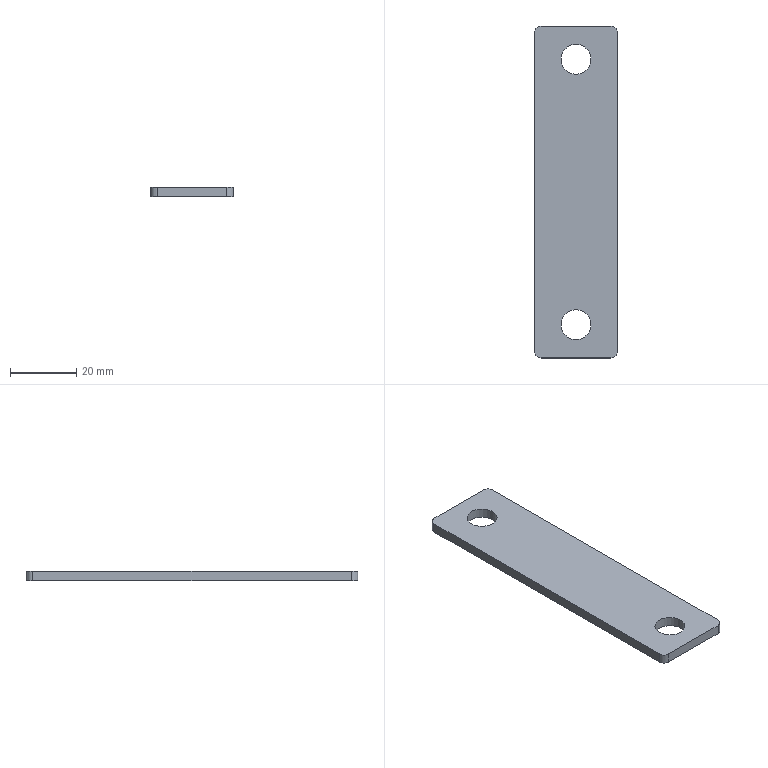Part | STEP file | 7471302 | 1 solid | 12 faces | box 25 x 100 x 3 mm | volume 7108 mm3 | cylinder 6 | plane 6 | commonest cylinder face diameters 4 x4 9 x2
STEP:
#1=CARTESIAN_POINT('',(0.,0.,0.));
#2=DIRECTION('',(0.,0.,1.));
#3=DIRECTION('',(1.,0.,0.));
#4=AXIS2_PLACEMENT_3D('',#1,#2,#3);
#5=CARTESIAN_POINT('',(15.714,-68.195,0.));
#6=VERTEX_POINT('',#5);
#7=CARTESIAN_POINT('',(17.714,-66.195,0.));
#8=VERTEX_POINT('',#7);
#9=CARTESIAN_POINT('',(15.714,-66.195,0.));
#10=DIRECTION('',(0.,0.,1.));
#11=DIRECTION('',(1.,0.,0.));
#12=AXIS2_PLACEMENT_3D('',#9,#10,#11);
#13=CIRCLE('',#12,2.);
#14=CARTESIAN_POINT('',(15.714,-66.195,3.));
#15=DIRECTION('',(0.,0.,-1.));
#16=DIRECTION('',(-1.,0.,0.));
#17=AXIS2_PLACEMENT_3D('',#14,#15,#16);
#18=CYLINDRICAL_SURFACE('',#17,2.);
#19=CARTESIAN_POINT('',(9.425,3.));
#20=DIRECTION('',(-1.,0.));
#21=VECTOR('',#20,1.);
#22=LINE('',#19,#21);
#23=(GEOMETRIC_REPRESENTATION_CONTEXT(2)PARAMETRIC_REPRESENTATION_CONTEXT()REPRESENTATION_CONTEXT('',''));
#24=DEFINITIONAL_REPRESENTATION('',(#22),#23);
#25=PCURVE('',#18,#24);
#26=CARTESIAN_POINT('',(15.714,-66.195,0.));
#27=DIRECTION('',(0.,0.,1.));
#28=DIRECTION('',(1.,0.,0.));
#29=AXIS2_PLACEMENT_3D('',#26,#27,#28);
#30=PLANE('',#29);
#31=CARTESIAN_POINT('',(0.,0.));
#32=DIRECTION('',(1.,0.));
#33=AXIS2_PLACEMENT_2D('',#31,#32);
#34=CIRCLE('',#33,2.);
#35=(GEOMETRIC_REPRESENTATION_CONTEXT(2)PARAMETRIC_REPRESENTATION_CONTEXT()REPRESENTATION_CONTEXT('',''));
#36=DEFINITIONAL_REPRESENTATION('',(#34),#35);
#37=PCURVE('',#30,#36);
#38=SURFACE_CURVE('',#13,(#25,#37),.PCURVE_S1.);
#39=EDGE_CURVE('',#6,#8,#38,.T.);
#40=ORIENTED_EDGE('',*,*,#39,.T.);
#41=CARTESIAN_POINT('',(17.714,-66.195,3.));
#42=VERTEX_POINT('',#41);
#43=CARTESIAN_POINT('',(17.714,-66.195,3.));
#44=DIRECTION('',(0.,0.,-1.));
#45=VECTOR('',#44,1.);
#46=LINE('',#43,#45);
#47=CARTESIAN_POINT('',(3.142,0.));
#48=DIRECTION('',(0.,1.));
#49=VECTOR('',#48,1.);
#50=LINE('',#47,#49);
#51=(GEOMETRIC_REPRESENTATION_CONTEXT(2)PARAMETRIC_REPRESENTATION_CONTEXT()REPRESENTATION_CONTEXT('',''));
#52=DEFINITIONAL_REPRESENTATION('',(#50),#51);
#53=PCURVE('',#18,#52);
#54=CARTESIAN_POINT('',(17.714,29.805,3.));
#55=DIRECTION('',(-1.,0.,0.));
#56=DIRECTION('',(0.,-1.,0.));
#57=AXIS2_PLACEMENT_3D('',#54,#55,#56);
#58=PLANE('',#57);
#59=CARTESIAN_POINT('',(96.,0.));
#60=DIRECTION('',(0.,-1.));
#61=VECTOR('',#60,1.);
#62=LINE('',#59,#61);
#63=(GEOMETRIC_REPRESENTATION_CONTEXT(2)PARAMETRIC_REPRESENTATION_CONTEXT()REPRESENTATION_CONTEXT('',''));
#64=DEFINITIONAL_REPRESENTATION('',(#62),#63);
#65=PCURVE('',#58,#64);
#66=SURFACE_CURVE('',#46,(#53,#65),.PCURVE_S1.);
#67=EDGE_CURVE('',#42,#8,#66,.T.);
#68=ORIENTED_EDGE('',*,*,#67,.F.);
#69=CARTESIAN_POINT('',(15.714,-68.195,3.));
#70=VERTEX_POINT('',#69);
#71=CARTESIAN_POINT('',(15.714,-66.195,3.));
#72=DIRECTION('',(0.,0.,1.));
#73=DIRECTION('',(1.,0.,0.));
#74=AXIS2_PLACEMENT_3D('',#71,#72,#73);
#75=CIRCLE('',#74,2.);
#76=CARTESIAN_POINT('',(9.425,0.));
#77=DIRECTION('',(-1.,0.));
#78=VECTOR('',#77,1.);
#79=LINE('',#76,#78);
#80=(GEOMETRIC_REPRESENTATION_CONTEXT(2)PARAMETRIC_REPRESENTATION_CONTEXT()REPRESENTATION_CONTEXT('',''));
#81=DEFINITIONAL_REPRESENTATION('',(#79),#80);
#82=PCURVE('',#18,#81);
#83=CARTESIAN_POINT('',(15.714,-66.195,3.));
#84=DIRECTION('',(0.,0.,1.));
#85=DIRECTION('',(1.,0.,0.));
#86=AXIS2_PLACEMENT_3D('',#83,#84,#85);
#87=PLANE('',#86);
#88=CARTESIAN_POINT('',(0.,0.));
#89=DIRECTION('',(1.,0.));
#90=AXIS2_PLACEMENT_2D('',#88,#89);
#91=CIRCLE('',#90,2.);
#92=(GEOMETRIC_REPRESENTATION_CONTEXT(2)PARAMETRIC_REPRESENTATION_CONTEXT()REPRESENTATION_CONTEXT('',''));
#93=DEFINITIONAL_REPRESENTATION('',(#91),#92);
#94=PCURVE('',#87,#93);
#95=SURFACE_CURVE('',#75,(#82,#94),.PCURVE_S1.);
#96=EDGE_CURVE('',#70,#42,#95,.T.);
#97=ORIENTED_EDGE('',*,*,#96,.F.);
#98=CARTESIAN_POINT('',(15.714,-68.195,3.));
#99=DIRECTION('',(0.,0.,-1.));
#100=VECTOR('',#99,1.);
#101=LINE('',#98,#100);
#102=CARTESIAN_POINT('',(4.712,0.));
#103=DIRECTION('',(0.,1.));
#104=VECTOR('',#103,1.);
#105=LINE('',#102,#104);
#106=(GEOMETRIC_REPRESENTATION_CONTEXT(2)PARAMETRIC_REPRESENTATION_CONTEXT()REPRESENTATION_CONTEXT('',''));
#107=DEFINITIONAL_REPRESENTATION('',(#105),#106);
#108=PCURVE('',#18,#107);
#109=CARTESIAN_POINT('',(-5.286,-68.195,3.));
#110=DIRECTION('',(0.,1.,0.));
#111=DIRECTION('',(0.,0.,1.));
#112=AXIS2_PLACEMENT_3D('',#109,#110,#111);
#113=PLANE('',#112);
#114=CARTESIAN_POINT('',(0.,21.));
#115=DIRECTION('',(-1.,0.));
#116=VECTOR('',#115,1.);
#117=LINE('',#114,#116);
#118=(GEOMETRIC_REPRESENTATION_CONTEXT(2)PARAMETRIC_REPRESENTATION_CONTEXT()REPRESENTATION_CONTEXT('',''));
#119=DEFINITIONAL_REPRESENTATION('',(#117),#118);
#120=PCURVE('',#113,#119);
#121=SURFACE_CURVE('',#101,(#108,#120),.PCURVE_S1.);
#122=EDGE_CURVE('',#70,#6,#121,.T.);
#123=ORIENTED_EDGE('',*,*,#122,.T.);
#124=EDGE_LOOP('',(#40,#68,#97,#123));
#125=FACE_BOUND('',#124,.T.);
#126=ADVANCED_FACE('',(#125),#18,.T.);
#127=CARTESIAN_POINT('',(17.714,29.805,0.));
#128=VERTEX_POINT('',#127);
#129=CARTESIAN_POINT('',(17.714,29.805,0.));
#130=DIRECTION('',(0.,1.,0.));
#131=VECTOR('',#130,1.);
#132=LINE('',#129,#131);
#133=CARTESIAN_POINT('',(0.,-3.));
#134=DIRECTION('',(-1.,0.));
#135=VECTOR('',#134,1.);
#136=LINE('',#133,#135);
#137=(GEOMETRIC_REPRESENTATION_CONTEXT(2)PARAMETRIC_REPRESENTATION_CONTEXT()REPRESENTATION_CONTEXT('',''));
#138=DEFINITIONAL_REPRESENTATION('',(#136),#137);
#139=PCURVE('',#58,#138);
#140=CARTESIAN_POINT('',(2.,96.));
#141=DIRECTION('',(0.,1.));
#142=VECTOR('',#141,1.);
#143=LINE('',#140,#142);
#144=(GEOMETRIC_REPRESENTATION_CONTEXT(2)PARAMETRIC_REPRESENTATION_CONTEXT()REPRESENTATION_CONTEXT('',''));
#145=DEFINITIONAL_REPRESENTATION('',(#143),#144);
#146=PCURVE('',#30,#145);
#147=SURFACE_CURVE('',#132,(#139,#146),.PCURVE_S1.);
#148=EDGE_CURVE('',#8,#128,#147,.T.);
#149=ORIENTED_EDGE('',*,*,#148,.T.);
#150=CARTESIAN_POINT('',(17.714,29.805,3.));
#151=VERTEX_POINT('',#150);
#152=CARTESIAN_POINT('',(17.714,29.805,3.));
#153=DIRECTION('',(0.,0.,-1.));
#154=VECTOR('',#153,1.);
#155=LINE('',#152,#154);
#156=CARTESIAN_POINT('',(0.,0.));
#157=DIRECTION('',(0.,-1.));
#158=VECTOR('',#157,1.);
#159=LINE('',#156,#158);
#160=(GEOMETRIC_REPRESENTATION_CONTEXT(2)PARAMETRIC_REPRESENTATION_CONTEXT()REPRESENTATION_CONTEXT('',''));
#161=DEFINITIONAL_REPRESENTATION('',(#159),#160);
#162=PCURVE('',#58,#161);
#163=CARTESIAN_POINT('',(15.714,29.805,3.));
#164=DIRECTION('',(0.,0.,-1.));
#165=DIRECTION('',(-1.,0.,0.));
#166=AXIS2_PLACEMENT_3D('',#163,#164,#165);
#167=CYLINDRICAL_SURFACE('',#166,2.);
#168=CARTESIAN_POINT('',(3.142,0.));
#169=DIRECTION('',(0.,1.));
#170=VECTOR('',#169,1.);
#171=LINE('',#168,#170);
#172=(GEOMETRIC_REPRESENTATION_CONTEXT(2)PARAMETRIC_REPRESENTATION_CONTEXT()REPRESENTATION_CONTEXT('',''));
#173=DEFINITIONAL_REPRESENTATION('',(#171),#172);
#174=PCURVE('',#167,#173);
#175=SURFACE_CURVE('',#155,(#162,#174),.PCURVE_S1.);
#176=EDGE_CURVE('',#151,#128,#175,.T.);
#177=ORIENTED_EDGE('',*,*,#176,.F.);
#178=CARTESIAN_POINT('',(17.714,29.805,3.));
#179=DIRECTION('',(0.,1.,0.));
#180=VECTOR('',#179,1.);
#181=LINE('',#178,#180);
#182=CARTESIAN_POINT('',(0.,0.));
#183=DIRECTION('',(-1.,0.));
#184=VECTOR('',#183,1.);
#185=LINE('',#182,#184);
#186=(GEOMETRIC_REPRESENTATION_CONTEXT(2)PARAMETRIC_REPRESENTATION_CONTEXT()REPRESENTATION_CONTEXT('',''));
#187=DEFINITIONAL_REPRESENTATION('',(#185),#186);
#188=PCURVE('',#58,#187);
#189=CARTESIAN_POINT('',(2.,96.));
#190=DIRECTION('',(0.,1.));
#191=VECTOR('',#190,1.);
#192=LINE('',#189,#191);
#193=(GEOMETRIC_REPRESENTATION_CONTEXT(2)PARAMETRIC_REPRESENTATION_CONTEXT()REPRESENTATION_CONTEXT('',''));
#194=DEFINITIONAL_REPRESENTATION('',(#192),#193);
#195=PCURVE('',#87,#194);
#196=SURFACE_CURVE('',#181,(#188,#195),.PCURVE_S1.);
#197=EDGE_CURVE('',#42,#151,#196,.T.);
#198=ORIENTED_EDGE('',*,*,#197,.F.);
#199=ORIENTED_EDGE('',*,*,#67,.T.);
#200=EDGE_LOOP('',(#149,#177,#198,#199));
#201=FACE_BOUND('',#200,.T.);
#202=ADVANCED_FACE('',(#201),#58,.F.);
#203=CARTESIAN_POINT('',(15.714,31.805,0.));
#204=VERTEX_POINT('',#203);
#205=CARTESIAN_POINT('',(15.714,29.805,0.));
#206=DIRECTION('',(0.,0.,1.));
#207=DIRECTION('',(-1.,0.,0.));
#208=AXIS2_PLACEMENT_3D('',#205,#206,#207);
#209=CIRCLE('',#208,2.);
#210=CARTESIAN_POINT('',(6.283,3.));
#211=DIRECTION('',(-1.,0.));
#212=VECTOR('',#211,1.);
#213=LINE('',#210,#212);
#214=(GEOMETRIC_REPRESENTATION_CONTEXT(2)PARAMETRIC_REPRESENTATION_CONTEXT()REPRESENTATION_CONTEXT('',''));
#215=DEFINITIONAL_REPRESENTATION('',(#213),#214);
#216=PCURVE('',#167,#215);
#217=CARTESIAN_POINT('',(0.,96.));
#218=DIRECTION('',(-1.,0.));
#219=AXIS2_PLACEMENT_2D('',#217,#218);
#220=CIRCLE('',#219,2.);
#221=(GEOMETRIC_REPRESENTATION_CONTEXT(2)PARAMETRIC_REPRESENTATION_CONTEXT()REPRESENTATION_CONTEXT('',''));
#222=DEFINITIONAL_REPRESENTATION('',(#220),#221);
#223=PCURVE('',#30,#222);
#224=SURFACE_CURVE('',#209,(#216,#223),.PCURVE_S1.);
#225=EDGE_CURVE('',#128,#204,#224,.T.);
#226=ORIENTED_EDGE('',*,*,#225,.T.);
#227=CARTESIAN_POINT('',(15.714,31.805,3.));
#228=VERTEX_POINT('',#227);
#229=CARTESIAN_POINT('',(15.714,31.805,3.));
#230=DIRECTION('',(0.,0.,-1.));
#231=VECTOR('',#230,1.);
#232=LINE('',#229,#231);
#233=CARTESIAN_POINT('',(1.571,0.));
#234=DIRECTION('',(0.,1.));
#235=VECTOR('',#234,1.);
#236=LINE('',#233,#235);
#237=(GEOMETRIC_REPRESENTATION_CONTEXT(2)PARAMETRIC_REPRESENTATION_CONTEXT()REPRESENTATION_CONTEXT('',''));
#238=DEFINITIONAL_REPRESENTATION('',(#236),#237);
#239=PCURVE('',#167,#238);
#240=CARTESIAN_POINT('',(-5.286,31.805,3.));
#241=DIRECTION('',(0.,-1.,0.));
#242=DIRECTION('',(0.,0.,-1.));
#243=AXIS2_PLACEMENT_3D('',#240,#241,#242);
#244=PLANE('',#243);
#245=CARTESIAN_POINT('',(0.,21.));
#246=DIRECTION('',(1.,0.));
#247=VECTOR('',#246,1.);
#248=LINE('',#245,#247);
#249=(GEOMETRIC_REPRESENTATION_CONTEXT(2)PARAMETRIC_REPRESENTATION_CONTEXT()REPRESENTATION_CONTEXT('',''));
#250=DEFINITIONAL_REPRESENTATION('',(#248),#249);
#251=PCURVE('',#244,#250);
#252=SURFACE_CURVE('',#232,(#239,#251),.PCURVE_S1.);
#253=EDGE_CURVE('',#228,#204,#252,.T.);
#254=ORIENTED_EDGE('',*,*,#253,.F.);
#255=CARTESIAN_POINT('',(15.714,29.805,3.));
#256=DIRECTION('',(0.,0.,1.));
#257=DIRECTION('',(-1.,0.,0.));
#258=AXIS2_PLACEMENT_3D('',#255,#256,#257);
#259=CIRCLE('',#258,2.);
#260=CARTESIAN_POINT('',(6.283,0.));
#261=DIRECTION('',(-1.,0.));
#262=VECTOR('',#261,1.);
#263=LINE('',#260,#262);
#264=(GEOMETRIC_REPRESENTATION_CONTEXT(2)PARAMETRIC_REPRESENTATION_CONTEXT()REPRESENTATION_CONTEXT('',''));
#265=DEFINITIONAL_REPRESENTATION('',(#263),#264);
#266=PCURVE('',#167,#265);
#267=CARTESIAN_POINT('',(0.,96.));
#268=DIRECTION('',(-1.,0.));
#269=AXIS2_PLACEMENT_2D('',#267,#268);
#270=CIRCLE('',#269,2.);
#271=(GEOMETRIC_REPRESENTATION_CONTEXT(2)PARAMETRIC_REPRESENTATION_CONTEXT()REPRESENTATION_CONTEXT('',''));
#272=DEFINITIONAL_REPRESENTATION('',(#270),#271);
#273=PCURVE('',#87,#272);
#274=SURFACE_CURVE('',#259,(#266,#273),.PCURVE_S1.);
#275=EDGE_CURVE('',#151,#228,#274,.T.);
#276=ORIENTED_EDGE('',*,*,#275,.F.);
#277=ORIENTED_EDGE('',*,*,#176,.T.);
#278=EDGE_LOOP('',(#226,#254,#276,#277));
#279=FACE_BOUND('',#278,.T.);
#280=ADVANCED_FACE('',(#279),#167,.T.);
#281=CARTESIAN_POINT('',(-5.286,31.805,0.));
#282=VERTEX_POINT('',#281);
#283=CARTESIAN_POINT('',(-5.286,31.805,0.));
#284=DIRECTION('',(-1.,0.,0.));
#285=VECTOR('',#284,1.);
#286=LINE('',#283,#285);
#287=CARTESIAN_POINT('',(3.,0.));
#288=DIRECTION('',(0.,-1.));
#289=VECTOR('',#288,1.);
#290=LINE('',#287,#289);
#291=(GEOMETRIC_REPRESENTATION_CONTEXT(2)PARAMETRIC_REPRESENTATION_CONTEXT()REPRESENTATION_CONTEXT('',''));
#292=DEFINITIONAL_REPRESENTATION('',(#290),#291);
#293=PCURVE('',#244,#292);
#294=CARTESIAN_POINT('',(-21.,98.));
#295=DIRECTION('',(-1.,0.));
#296=VECTOR('',#295,1.);
#297=LINE('',#294,#296);
#298=(GEOMETRIC_REPRESENTATION_CONTEXT(2)PARAMETRIC_REPRESENTATION_CONTEXT()REPRESENTATION_CONTEXT('',''));
#299=DEFINITIONAL_REPRESENTATION('',(#297),#298);
#300=PCURVE('',#30,#299);
#301=SURFACE_CURVE('',#286,(#293,#300),.PCURVE_S1.);
#302=EDGE_CURVE('',#204,#282,#301,.T.);
#303=ORIENTED_EDGE('',*,*,#302,.T.);
#304=CARTESIAN_POINT('',(-5.286,31.805,3.));
#305=VERTEX_POINT('',#304);
#306=CARTESIAN_POINT('',(-5.286,31.805,3.));
#307=DIRECTION('',(0.,0.,-1.));
#308=VECTOR('',#307,1.);
#309=LINE('',#306,#308);
#310=CARTESIAN_POINT('',(0.,0.));
#311=DIRECTION('',(1.,0.));
#312=VECTOR('',#311,1.);
#313=LINE('',#310,#312);
#314=(GEOMETRIC_REPRESENTATION_CONTEXT(2)PARAMETRIC_REPRESENTATION_CONTEXT()REPRESENTATION_CONTEXT('',''));
#315=DEFINITIONAL_REPRESENTATION('',(#313),#314);
#316=PCURVE('',#244,#315);
#317=CARTESIAN_POINT('',(-5.286,29.805,3.));
#318=DIRECTION('',(0.,0.,-1.));
#319=DIRECTION('',(-1.,0.,0.));
#320=AXIS2_PLACEMENT_3D('',#317,#318,#319);
#321=CYLINDRICAL_SURFACE('',#320,2.);
#322=CARTESIAN_POINT('',(1.571,0.));
#323=DIRECTION('',(0.,1.));
#324=VECTOR('',#323,1.);
#325=LINE('',#322,#324);
#326=(GEOMETRIC_REPRESENTATION_CONTEXT(2)PARAMETRIC_REPRESENTATION_CONTEXT()REPRESENTATION_CONTEXT('',''));
#327=DEFINITIONAL_REPRESENTATION('',(#325),#326);
#328=PCURVE('',#321,#327);
#329=SURFACE_CURVE('',#309,(#316,#328),.PCURVE_S1.);
#330=EDGE_CURVE('',#305,#282,#329,.T.);
#331=ORIENTED_EDGE('',*,*,#330,.F.);
#332=CARTESIAN_POINT('',(-5.286,31.805,3.));
#333=DIRECTION('',(-1.,0.,0.));
#334=VECTOR('',#333,1.);
#335=LINE('',#332,#334);
#336=CARTESIAN_POINT('',(0.,0.));
#337=DIRECTION('',(0.,-1.));
#338=VECTOR('',#337,1.);
#339=LINE('',#336,#338);
#340=(GEOMETRIC_REPRESENTATION_CONTEXT(2)PARAMETRIC_REPRESENTATION_CONTEXT()REPRESENTATION_CONTEXT('',''));
#341=DEFINITIONAL_REPRESENTATION('',(#339),#340);
#342=PCURVE('',#244,#341);
#343=CARTESIAN_POINT('',(-21.,98.));
#344=DIRECTION('',(-1.,0.));
#345=VECTOR('',#344,1.);
#346=LINE('',#343,#345);
#347=(GEOMETRIC_REPRESENTATION_CONTEXT(2)PARAMETRIC_REPRESENTATION_CONTEXT()REPRESENTATION_CONTEXT('',''));
#348=DEFINITIONAL_REPRESENTATION('',(#346),#347);
#349=PCURVE('',#87,#348);
#350=SURFACE_CURVE('',#335,(#342,#349),.PCURVE_S1.);
#351=EDGE_CURVE('',#228,#305,#350,.T.);
#352=ORIENTED_EDGE('',*,*,#351,.F.);
#353=ORIENTED_EDGE('',*,*,#253,.T.);
#354=EDGE_LOOP('',(#303,#331,#352,#353));
#355=FACE_BOUND('',#354,.T.);
#356=ADVANCED_FACE('',(#355),#244,.F.);
#357=CARTESIAN_POINT('',(-7.286,29.805,0.));
#358=VERTEX_POINT('',#357);
#359=CARTESIAN_POINT('',(-5.286,29.805,0.));
#360=DIRECTION('',(0.,0.,1.));
#361=DIRECTION('',(1.,0.,0.));
#362=AXIS2_PLACEMENT_3D('',#359,#360,#361);
#363=CIRCLE('',#362,2.);
#364=CARTESIAN_POINT('',(3.142,3.));
#365=DIRECTION('',(-1.,0.));
#366=VECTOR('',#365,1.);
#367=LINE('',#364,#366);
#368=(GEOMETRIC_REPRESENTATION_CONTEXT(2)PARAMETRIC_REPRESENTATION_CONTEXT()REPRESENTATION_CONTEXT('',''));
#369=DEFINITIONAL_REPRESENTATION('',(#367),#368);
#370=PCURVE('',#321,#369);
#371=CARTESIAN_POINT('',(-21.,96.));
#372=DIRECTION('',(1.,0.));
#373=AXIS2_PLACEMENT_2D('',#371,#372);
#374=CIRCLE('',#373,2.);
#375=(GEOMETRIC_REPRESENTATION_CONTEXT(2)PARAMETRIC_REPRESENTATION_CONTEXT()REPRESENTATION_CONTEXT('',''));
#376=DEFINITIONAL_REPRESENTATION('',(#374),#375);
#377=PCURVE('',#30,#376);
#378=SURFACE_CURVE('',#363,(#370,#377),.PCURVE_S1.);
#379=EDGE_CURVE('',#282,#358,#378,.T.);
#380=ORIENTED_EDGE('',*,*,#379,.T.);
#381=CARTESIAN_POINT('',(-7.286,29.805,3.));
#382=VERTEX_POINT('',#381);
#383=CARTESIAN_POINT('',(-7.286,29.805,3.));
#384=DIRECTION('',(0.,0.,-1.));
#385=VECTOR('',#384,1.);
#386=LINE('',#383,#385);
#387=CARTESIAN_POINT('',(0.,0.));
#388=DIRECTION('',(0.,1.));
#389=VECTOR('',#388,1.);
#390=LINE('',#387,#389);
#391=(GEOMETRIC_REPRESENTATION_CONTEXT(2)PARAMETRIC_REPRESENTATION_CONTEXT()REPRESENTATION_CONTEXT('',''));
#392=DEFINITIONAL_REPRESENTATION('',(#390),#391);
#393=PCURVE('',#321,#392);
#394=CARTESIAN_POINT('',(-7.286,29.805,3.));
#395=DIRECTION('',(1.,0.,0.));
#396=DIRECTION('',(0.,1.,0.));
#397=AXIS2_PLACEMENT_3D('',#394,#395,#396);
#398=PLANE('',#397);
#399=CARTESIAN_POINT('',(0.,0.));
#400=DIRECTION('',(0.,-1.));
#401=VECTOR('',#400,1.);
#402=LINE('',#399,#401);
#403=(GEOMETRIC_REPRESENTATION_CONTEXT(2)PARAMETRIC_REPRESENTATION_CONTEXT()REPRESENTATION_CONTEXT('',''));
#404=DEFINITIONAL_REPRESENTATION('',(#402),#403);
#405=PCURVE('',#398,#404);
#406=SURFACE_CURVE('',#386,(#393,#405),.PCURVE_S1.);
#407=EDGE_CURVE('',#382,#358,#406,.T.);
#408=ORIENTED_EDGE('',*,*,#407,.F.);
#409=CARTESIAN_POINT('',(-5.286,29.805,3.));
#410=DIRECTION('',(0.,0.,1.));
#411=DIRECTION('',(1.,0.,0.));
#412=AXIS2_PLACEMENT_3D('',#409,#410,#411);
#413=CIRCLE('',#412,2.);
#414=CARTESIAN_POINT('',(3.142,0.));
#415=DIRECTION('',(-1.,0.));
#416=VECTOR('',#415,1.);
#417=LINE('',#414,#416);
#418=(GEOMETRIC_REPRESENTATION_CONTEXT(2)PARAMETRIC_REPRESENTATION_CONTEXT()REPRESENTATION_CONTEXT('',''));
#419=DEFINITIONAL_REPRESENTATION('',(#417),#418);
#420=PCURVE('',#321,#419);
#421=CARTESIAN_POINT('',(-21.,96.));
#422=DIRECTION('',(1.,0.));
#423=AXIS2_PLACEMENT_2D('',#421,#422);
#424=CIRCLE('',#423,2.);
#425=(GEOMETRIC_REPRESENTATION_CONTEXT(2)PARAMETRIC_REPRESENTATION_CONTEXT()REPRESENTATION_CONTEXT('',''));
#426=DEFINITIONAL_REPRESENTATION('',(#424),#425);
#427=PCURVE('',#87,#426);
#428=SURFACE_CURVE('',#413,(#420,#427),.PCURVE_S1.);
#429=EDGE_CURVE('',#305,#382,#428,.T.);
#430=ORIENTED_EDGE('',*,*,#429,.F.);
#431=ORIENTED_EDGE('',*,*,#330,.T.);
#432=EDGE_LOOP('',(#380,#408,#430,#431));
#433=FACE_BOUND('',#432,.T.);
#434=ADVANCED_FACE('',(#433),#321,.T.);
#435=CARTESIAN_POINT('',(-7.286,-66.195,0.));
#436=VERTEX_POINT('',#435);
#437=CARTESIAN_POINT('',(-7.286,29.805,0.));
#438=DIRECTION('',(0.,-1.,0.));
#439=VECTOR('',#438,1.);
#440=LINE('',#437,#439);
#441=CARTESIAN_POINT('',(0.,-3.));
#442=DIRECTION('',(-1.,0.));
#443=VECTOR('',#442,1.);
#444=LINE('',#441,#443);
#445=(GEOMETRIC_REPRESENTATION_CONTEXT(2)PARAMETRIC_REPRESENTATION_CONTEXT()REPRESENTATION_CONTEXT('',''));
#446=DEFINITIONAL_REPRESENTATION('',(#444),#445);
#447=PCURVE('',#398,#446);
#448=CARTESIAN_POINT('',(-23.,96.));
#449=DIRECTION('',(0.,-1.));
#450=VECTOR('',#449,1.);
#451=LINE('',#448,#450);
#452=(GEOMETRIC_REPRESENTATION_CONTEXT(2)PARAMETRIC_REPRESENTATION_CONTEXT()REPRESENTATION_CONTEXT('',''));
#453=DEFINITIONAL_REPRESENTATION('',(#451),#452);
#454=PCURVE('',#30,#453);
#455=SURFACE_CURVE('',#440,(#447,#454),.PCURVE_S1.);
#456=EDGE_CURVE('',#358,#436,#455,.T.);
#457=ORIENTED_EDGE('',*,*,#456,.T.);
#458=CARTESIAN_POINT('',(-7.286,-66.195,3.));
#459=VERTEX_POINT('',#458);
#460=CARTESIAN_POINT('',(-7.286,-66.195,3.));
#461=DIRECTION('',(0.,0.,-1.));
#462=VECTOR('',#461,1.);
#463=LINE('',#460,#462);
#464=CARTESIAN_POINT('',(-96.,0.));
#465=DIRECTION('',(0.,-1.));
#466=VECTOR('',#465,1.);
#467=LINE('',#464,#466);
#468=(GEOMETRIC_REPRESENTATION_CONTEXT(2)PARAMETRIC_REPRESENTATION_CONTEXT()REPRESENTATION_CONTEXT('',''));
#469=DEFINITIONAL_REPRESENTATION('',(#467),#468);
#470=PCURVE('',#398,#469);
#471=CARTESIAN_POINT('',(-5.286,-66.195,3.));
#472=DIRECTION('',(0.,0.,-1.));
#473=DIRECTION('',(-1.,0.,0.));
#474=AXIS2_PLACEMENT_3D('',#471,#472,#473);
#475=CYLINDRICAL_SURFACE('',#474,2.);
#476=CARTESIAN_POINT('',(6.283,0.));
#477=DIRECTION('',(0.,1.));
#478=VECTOR('',#477,1.);
#479=LINE('',#476,#478);
#480=(GEOMETRIC_REPRESENTATION_CONTEXT(2)PARAMETRIC_REPRESENTATION_CONTEXT()REPRESENTATION_CONTEXT('',''));
#481=DEFINITIONAL_REPRESENTATION('',(#479),#480);
#482=PCURVE('',#475,#481);
#483=SURFACE_CURVE('',#463,(#470,#482),.PCURVE_S1.);
#484=EDGE_CURVE('',#459,#436,#483,.T.);
#485=ORIENTED_EDGE('',*,*,#484,.F.);
#486=CARTESIAN_POINT('',(-7.286,29.805,3.));
#487=DIRECTION('',(0.,-1.,0.));
#488=VECTOR('',#487,1.);
#489=LINE('',#486,#488);
#490=CARTESIAN_POINT('',(0.,0.));
#491=DIRECTION('',(-1.,0.));
#492=VECTOR('',#491,1.);
#493=LINE('',#490,#492);
#494=(GEOMETRIC_REPRESENTATION_CONTEXT(2)PARAMETRIC_REPRESENTATION_CONTEXT()REPRESENTATION_CONTEXT('',''));
#495=DEFINITIONAL_REPRESENTATION('',(#493),#494);
#496=PCURVE('',#398,#495);
#497=CARTESIAN_POINT('',(-23.,96.));
#498=DIRECTION('',(0.,-1.));
#499=VECTOR('',#498,1.);
#500=LINE('',#497,#499);
#501=(GEOMETRIC_REPRESENTATION_CONTEXT(2)PARAMETRIC_REPRESENTATION_CONTEXT()REPRESENTATION_CONTEXT('',''));
#502=DEFINITIONAL_REPRESENTATION('',(#500),#501);
#503=PCURVE('',#87,#502);
#504=SURFACE_CURVE('',#489,(#496,#503),.PCURVE_S1.);
#505=EDGE_CURVE('',#382,#459,#504,.T.);
#506=ORIENTED_EDGE('',*,*,#505,.F.);
#507=ORIENTED_EDGE('',*,*,#407,.T.);
#508=EDGE_LOOP('',(#457,#485,#506,#507));
#509=FACE_BOUND('',#508,.T.);
#510=ADVANCED_FACE('',(#509),#398,.F.);
#511=CARTESIAN_POINT('',(-5.286,-68.195,0.));
#512=VERTEX_POINT('',#511);
#513=CARTESIAN_POINT('',(-5.286,-66.195,0.));
#514=DIRECTION('',(0.,0.,1.));
#515=DIRECTION('',(1.,0.,0.));
#516=AXIS2_PLACEMENT_3D('',#513,#514,#515);
#517=CIRCLE('',#516,2.);
#518=CARTESIAN_POINT('',(9.425,3.));
#519=DIRECTION('',(-1.,0.));
#520=VECTOR('',#519,1.);
#521=LINE('',#518,#520);
#522=(GEOMETRIC_REPRESENTATION_CONTEXT(2)PARAMETRIC_REPRESENTATION_CONTEXT()REPRESENTATION_CONTEXT('',''));
#523=DEFINITIONAL_REPRESENTATION('',(#521),#522);
#524=PCURVE('',#475,#523);
#525=CARTESIAN_POINT('',(-21.,0.));
#526=DIRECTION('',(1.,0.));
#527=AXIS2_PLACEMENT_2D('',#525,#526);
#528=CIRCLE('',#527,2.);
#529=(GEOMETRIC_REPRESENTATION_CONTEXT(2)PARAMETRIC_REPRESENTATION_CONTEXT()REPRESENTATION_CONTEXT('',''));
#530=DEFINITIONAL_REPRESENTATION('',(#528),#529);
#531=PCURVE('',#30,#530);
#532=SURFACE_CURVE('',#517,(#524,#531),.PCURVE_S1.);
#533=EDGE_CURVE('',#436,#512,#532,.T.);
#534=ORIENTED_EDGE('',*,*,#533,.T.);
#535=CARTESIAN_POINT('',(-5.286,-68.195,3.));
#536=VERTEX_POINT('',#535);
#537=CARTESIAN_POINT('',(-5.286,-68.195,3.));
#538=DIRECTION('',(0.,0.,-1.));
#539=VECTOR('',#538,1.);
#540=LINE('',#537,#539);
#541=CARTESIAN_POINT('',(4.712,0.));
#542=DIRECTION('',(0.,1.));
#543=VECTOR('',#542,1.);
#544=LINE('',#541,#543);
#545=(GEOMETRIC_REPRESENTATION_CONTEXT(2)PARAMETRIC_REPRESENTATION_CONTEXT()REPRESENTATION_CONTEXT('',''));
#546=DEFINITIONAL_REPRESENTATION('',(#544),#545);
#547=PCURVE('',#475,#546);
#548=CARTESIAN_POINT('',(0.,0.));
#549=DIRECTION('',(-1.,0.));
#550=VECTOR('',#549,1.);
#551=LINE('',#548,#550);
#552=(GEOMETRIC_REPRESENTATION_CONTEXT(2)PARAMETRIC_REPRESENTATION_CONTEXT()REPRESENTATION_CONTEXT('',''));
#553=DEFINITIONAL_REPRESENTATION('',(#551),#552);
#554=PCURVE('',#113,#553);
#555=SURFACE_CURVE('',#540,(#547,#554),.PCURVE_S1.);
#556=EDGE_CURVE('',#536,#512,#555,.T.);
#557=ORIENTED_EDGE('',*,*,#556,.F.);
#558=CARTESIAN_POINT('',(-5.286,-66.195,3.));
#559=DIRECTION('',(0.,0.,1.));
#560=DIRECTION('',(1.,0.,0.));
#561=AXIS2_PLACEMENT_3D('',#558,#559,#560);
#562=CIRCLE('',#561,2.);
#563=CARTESIAN_POINT('',(9.425,0.));
#564=DIRECTION('',(-1.,0.));
#565=VECTOR('',#564,1.);
#566=LINE('',#563,#565);
#567=(GEOMETRIC_REPRESENTATION_CONTEXT(2)PARAMETRIC_REPRESENTATION_CONTEXT()REPRESENTATION_CONTEXT('',''));
#568=DEFINITIONAL_REPRESENTATION('',(#566),#567);
#569=PCURVE('',#475,#568);
#570=CARTESIAN_POINT('',(-21.,0.));
#571=DIRECTION('',(1.,0.));
#572=AXIS2_PLACEMENT_2D('',#570,#571);
#573=CIRCLE('',#572,2.);
#574=(GEOMETRIC_REPRESENTATION_CONTEXT(2)PARAMETRIC_REPRESENTATION_CONTEXT()REPRESENTATION_CONTEXT('',''));
#575=DEFINITIONAL_REPRESENTATION('',(#573),#574);
#576=PCURVE('',#87,#575);
#577=SURFACE_CURVE('',#562,(#569,#576),.PCURVE_S1.);
#578=EDGE_CURVE('',#459,#536,#577,.T.);
#579=ORIENTED_EDGE('',*,*,#578,.F.);
#580=ORIENTED_EDGE('',*,*,#484,.T.);
#581=EDGE_LOOP('',(#534,#557,#579,#580));
#582=FACE_BOUND('',#581,.T.);
#583=ADVANCED_FACE('',(#582),#475,.T.);
#584=CARTESIAN_POINT('',(-5.286,-68.195,0.));
#585=DIRECTION('',(1.,0.,0.));
#586=VECTOR('',#585,1.);
#587=LINE('',#584,#586);
#588=CARTESIAN_POINT('',(-3.,0.));
#589=DIRECTION('',(0.,1.));
#590=VECTOR('',#589,1.);
#591=LINE('',#588,#590);
#592=(GEOMETRIC_REPRESENTATION_CONTEXT(2)PARAMETRIC_REPRESENTATION_CONTEXT()REPRESENTATION_CONTEXT('',''));
#593=DEFINITIONAL_REPRESENTATION('',(#591),#592);
#594=PCURVE('',#113,#593);
#595=CARTESIAN_POINT('',(-21.,-2.));
#596=DIRECTION('',(1.,0.));
#597=VECTOR('',#596,1.);
#598=LINE('',#595,#597);
#599=(GEOMETRIC_REPRESENTATION_CONTEXT(2)PARAMETRIC_REPRESENTATION_CONTEXT()REPRESENTATION_CONTEXT('',''));
#600=DEFINITIONAL_REPRESENTATION('',(#598),#599);
#601=PCURVE('',#30,#600);
#602=SURFACE_CURVE('',#587,(#594,#601),.PCURVE_S1.);
#603=EDGE_CURVE('',#512,#6,#602,.T.);
#604=ORIENTED_EDGE('',*,*,#603,.T.);
#605=ORIENTED_EDGE('',*,*,#122,.F.);
#606=CARTESIAN_POINT('',(-5.286,-68.195,3.));
#607=DIRECTION('',(1.,0.,0.));
#608=VECTOR('',#607,1.);
#609=LINE('',#606,#608);
#610=CARTESIAN_POINT('',(0.,0.));
#611=DIRECTION('',(0.,1.));
#612=VECTOR('',#611,1.);
#613=LINE('',#610,#612);
#614=(GEOMETRIC_REPRESENTATION_CONTEXT(2)PARAMETRIC_REPRESENTATION_CONTEXT()REPRESENTATION_CONTEXT('',''));
#615=DEFINITIONAL_REPRESENTATION('',(#613),#614);
#616=PCURVE('',#113,#615);
#617=CARTESIAN_POINT('',(-21.,-2.));
#618=DIRECTION('',(1.,0.));
#619=VECTOR('',#618,1.);
#620=LINE('',#617,#619);
#621=(GEOMETRIC_REPRESENTATION_CONTEXT(2)PARAMETRIC_REPRESENTATION_CONTEXT()REPRESENTATION_CONTEXT('',''));
#622=DEFINITIONAL_REPRESENTATION('',(#620),#621);
#623=PCURVE('',#87,#622);
#624=SURFACE_CURVE('',#609,(#616,#623),.PCURVE_S1.);
#625=EDGE_CURVE('',#536,#70,#624,.T.);
#626=ORIENTED_EDGE('',*,*,#625,.F.);
#627=ORIENTED_EDGE('',*,*,#556,.T.);
#628=EDGE_LOOP('',(#604,#605,#626,#627));
#629=FACE_BOUND('',#628,.T.);
#630=ADVANCED_FACE('',(#629),#113,.F.);
#631=CARTESIAN_POINT('',(9.714,-58.195,3.));
#632=VERTEX_POINT('',#631);
#633=CARTESIAN_POINT('',(5.214,-58.195,3.));
#634=DIRECTION('',(0.,0.,1.));
#635=DIRECTION('',(1.,0.,0.));
#636=AXIS2_PLACEMENT_3D('',#633,#634,#635);
#637=CIRCLE('',#636,4.5);
#638=CARTESIAN_POINT('',(-10.5,8.));
#639=DIRECTION('',(1.,0.));
#640=AXIS2_PLACEMENT_2D('',#638,#639);
#641=CIRCLE('',#640,4.5);
#642=(GEOMETRIC_REPRESENTATION_CONTEXT(2)PARAMETRIC_REPRESENTATION_CONTEXT()REPRESENTATION_CONTEXT('',''));
#643=DEFINITIONAL_REPRESENTATION('',(#641),#642);
#644=PCURVE('',#87,#643);
#645=CARTESIAN_POINT('',(5.214,-58.195,0.));
#646=DIRECTION('',(0.,0.,1.));
#647=DIRECTION('',(1.,0.,0.));
#648=AXIS2_PLACEMENT_3D('',#645,#646,#647);
#649=CYLINDRICAL_SURFACE('',#648,4.5);
#650=CARTESIAN_POINT('',(0.,3.));
#651=DIRECTION('',(1.,0.));
#652=VECTOR('',#651,1.);
#653=LINE('',#650,#652);
#654=(GEOMETRIC_REPRESENTATION_CONTEXT(2)PARAMETRIC_REPRESENTATION_CONTEXT()REPRESENTATION_CONTEXT('',''));
#655=DEFINITIONAL_REPRESENTATION('',(#653),#654);
#656=PCURVE('',#649,#655);
#657=SURFACE_CURVE('',#637,(#644,#656),.PCURVE_S1.);
#658=EDGE_CURVE('',#632,#632,#657,.T.);
#659=ORIENTED_EDGE('',*,*,#658,.F.);
#660=EDGE_LOOP('',(#659));
#661=FACE_BOUND('',#660,.T.);
#662=CARTESIAN_POINT('',(9.714,21.805,3.));
#663=VERTEX_POINT('',#662);
#664=CARTESIAN_POINT('',(5.214,21.805,3.));
#665=DIRECTION('',(0.,0.,1.));
#666=DIRECTION('',(1.,0.,0.));
#667=AXIS2_PLACEMENT_3D('',#664,#665,#666);
#668=CIRCLE('',#667,4.5);
#669=CARTESIAN_POINT('',(-10.5,88.));
#670=DIRECTION('',(1.,0.));
#671=AXIS2_PLACEMENT_2D('',#669,#670);
#672=CIRCLE('',#671,4.5);
#673=(GEOMETRIC_REPRESENTATION_CONTEXT(2)PARAMETRIC_REPRESENTATION_CONTEXT()REPRESENTATION_CONTEXT('',''));
#674=DEFINITIONAL_REPRESENTATION('',(#672),#673);
#675=PCURVE('',#87,#674);
#676=CARTESIAN_POINT('',(5.214,21.805,0.));
#677=DIRECTION('',(0.,0.,1.));
#678=DIRECTION('',(1.,0.,0.));
#679=AXIS2_PLACEMENT_3D('',#676,#677,#678);
#680=CYLINDRICAL_SURFACE('',#679,4.5);
#681=CARTESIAN_POINT('',(0.,3.));
#682=DIRECTION('',(1.,0.));
#683=VECTOR('',#682,1.);
#684=LINE('',#681,#683);
#685=(GEOMETRIC_REPRESENTATION_CONTEXT(2)PARAMETRIC_REPRESENTATION_CONTEXT()REPRESENTATION_CONTEXT('',''));
#686=DEFINITIONAL_REPRESENTATION('',(#684),#685);
#687=PCURVE('',#680,#686);
#688=SURFACE_CURVE('',#668,(#675,#687),.PCURVE_S1.);
#689=EDGE_CURVE('',#663,#663,#688,.T.);
#690=ORIENTED_EDGE('',*,*,#689,.F.);
#691=EDGE_LOOP('',(#690));
#692=FACE_BOUND('',#691,.T.);
#693=ORIENTED_EDGE('',*,*,#96,.T.);
#694=ORIENTED_EDGE('',*,*,#197,.T.);
#695=ORIENTED_EDGE('',*,*,#275,.T.);
#696=ORIENTED_EDGE('',*,*,#351,.T.);
#697=ORIENTED_EDGE('',*,*,#429,.T.);
#698=ORIENTED_EDGE('',*,*,#505,.T.);
#699=ORIENTED_EDGE('',*,*,#578,.T.);
#700=ORIENTED_EDGE('',*,*,#625,.T.);
#701=EDGE_LOOP('',(#693,#694,#695,#696,#697,#698,#699,#700));
#702=FACE_BOUND('',#701,.T.);
#703=ADVANCED_FACE('',(#661,#692,#702),#87,.T.);
#704=CARTESIAN_POINT('',(9.714,-58.195,0.));
#705=VERTEX_POINT('',#704);
#706=CARTESIAN_POINT('',(5.214,-58.195,0.));
#707=DIRECTION('',(0.,0.,1.));
#708=DIRECTION('',(1.,0.,0.));
#709=AXIS2_PLACEMENT_3D('',#706,#707,#708);
#710=CIRCLE('',#709,4.5);
#711=CARTESIAN_POINT('',(-10.5,8.));
#712=DIRECTION('',(1.,0.));
#713=AXIS2_PLACEMENT_2D('',#711,#712);
#714=CIRCLE('',#713,4.5);
#715=(GEOMETRIC_REPRESENTATION_CONTEXT(2)PARAMETRIC_REPRESENTATION_CONTEXT()REPRESENTATION_CONTEXT('',''));
#716=DEFINITIONAL_REPRESENTATION('',(#714),#715);
#717=PCURVE('',#30,#716);
#718=CARTESIAN_POINT('',(0.,0.));
#719=DIRECTION('',(1.,0.));
#720=VECTOR('',#719,1.);
#721=LINE('',#718,#720);
#722=(GEOMETRIC_REPRESENTATION_CONTEXT(2)PARAMETRIC_REPRESENTATION_CONTEXT()REPRESENTATION_CONTEXT('',''));
#723=DEFINITIONAL_REPRESENTATION('',(#721),#722);
#724=PCURVE('',#649,#723);
#725=SURFACE_CURVE('',#710,(#717,#724),.PCURVE_S1.);
#726=EDGE_CURVE('',#705,#705,#725,.T.);
#727=ORIENTED_EDGE('',*,*,#726,.T.);
#728=EDGE_LOOP('',(#727));
#729=FACE_BOUND('',#728,.T.);
#730=CARTESIAN_POINT('',(9.714,21.805,0.));
#731=VERTEX_POINT('',#730);
#732=CARTESIAN_POINT('',(5.214,21.805,0.));
#733=DIRECTION('',(0.,0.,1.));
#734=DIRECTION('',(1.,0.,0.));
#735=AXIS2_PLACEMENT_3D('',#732,#733,#734);
#736=CIRCLE('',#735,4.5);
#737=CARTESIAN_POINT('',(-10.5,88.));
#738=DIRECTION('',(1.,0.));
#739=AXIS2_PLACEMENT_2D('',#737,#738);
#740=CIRCLE('',#739,4.5);
#741=(GEOMETRIC_REPRESENTATION_CONTEXT(2)PARAMETRIC_REPRESENTATION_CONTEXT()REPRESENTATION_CONTEXT('',''));
#742=DEFINITIONAL_REPRESENTATION('',(#740),#741);
#743=PCURVE('',#30,#742);
#744=CARTESIAN_POINT('',(0.,0.));
#745=DIRECTION('',(1.,0.));
#746=VECTOR('',#745,1.);
#747=LINE('',#744,#746);
#748=(GEOMETRIC_REPRESENTATION_CONTEXT(2)PARAMETRIC_REPRESENTATION_CONTEXT()REPRESENTATION_CONTEXT('',''));
#749=DEFINITIONAL_REPRESENTATION('',(#747),#748);
#750=PCURVE('',#680,#749);
#751=SURFACE_CURVE('',#736,(#743,#750),.PCURVE_S1.);
#752=EDGE_CURVE('',#731,#731,#751,.T.);
#753=ORIENTED_EDGE('',*,*,#752,.T.);
#754=EDGE_LOOP('',(#753));
#755=FACE_BOUND('',#754,.T.);
#756=ORIENTED_EDGE('',*,*,#39,.F.);
#757=ORIENTED_EDGE('',*,*,#603,.F.);
#758=ORIENTED_EDGE('',*,*,#533,.F.);
#759=ORIENTED_EDGE('',*,*,#456,.F.);
#760=ORIENTED_EDGE('',*,*,#379,.F.);
#761=ORIENTED_EDGE('',*,*,#302,.F.);
#762=ORIENTED_EDGE('',*,*,#225,.F.);
#763=ORIENTED_EDGE('',*,*,#148,.F.);
#764=EDGE_LOOP('',(#756,#757,#758,#759,#760,#761,#762,#763));
#765=FACE_BOUND('',#764,.T.);
#766=ADVANCED_FACE('',(#729,#755,#765),#30,.F.);
#767=ORIENTED_EDGE('',*,*,#752,.T.);
#768=CARTESIAN_POINT('',(9.714,21.805,0.));
#769=CARTESIAN_POINT('',(9.714,21.805,3.));
#770=B_SPLINE_CURVE_WITH_KNOTS('',1,(#768,#769),.UNSPECIFIED.,.F.,.F.,(2,2),(0.,3.),.PIECEWISE_BEZIER_KNOTS.);
#771=CARTESIAN_POINT('',(6.283,0.));
#772=DIRECTION('',(0.,1.));
#773=VECTOR('',#772,1.);
#774=LINE('',#771,#773);
#775=(GEOMETRIC_REPRESENTATION_CONTEXT(2)PARAMETRIC_REPRESENTATION_CONTEXT()REPRESENTATION_CONTEXT('',''));
#776=DEFINITIONAL_REPRESENTATION('',(#774),#775);
#777=PCURVE('',#680,#776);
#778=CARTESIAN_POINT('',(0.,0.));
#779=DIRECTION('',(0.,1.));
#780=VECTOR('',#779,1.);
#781=LINE('',#778,#780);
#782=(GEOMETRIC_REPRESENTATION_CONTEXT(2)PARAMETRIC_REPRESENTATION_CONTEXT()REPRESENTATION_CONTEXT('',''));
#783=DEFINITIONAL_REPRESENTATION('',(#781),#782);
#784=PCURVE('',#680,#783);
#785=SEAM_CURVE('',#770,(#777,#784),.PCURVE_S1.);
#786=EDGE_CURVE('',#731,#663,#785,.T.);
#787=ORIENTED_EDGE('',*,*,#786,.T.);
#788=ORIENTED_EDGE('',*,*,#689,.F.);
#789=ORIENTED_EDGE('',*,*,#786,.F.);
#790=EDGE_LOOP('',(#767,#787,#788,#789));
#791=FACE_BOUND('',#790,.F.);
#792=ADVANCED_FACE('',(#791),#680,.F.);
#793=ORIENTED_EDGE('',*,*,#726,.T.);
#794=CARTESIAN_POINT('',(9.714,-58.195,0.));
#795=CARTESIAN_POINT('',(9.714,-58.195,3.));
#796=B_SPLINE_CURVE_WITH_KNOTS('',1,(#794,#795),.UNSPECIFIED.,.F.,.F.,(2,2),(0.,3.),.PIECEWISE_BEZIER_KNOTS.);
#797=CARTESIAN_POINT('',(6.283,0.));
#798=DIRECTION('',(0.,1.));
#799=VECTOR('',#798,1.);
#800=LINE('',#797,#799);
#801=(GEOMETRIC_REPRESENTATION_CONTEXT(2)PARAMETRIC_REPRESENTATION_CONTEXT()REPRESENTATION_CONTEXT('',''));
#802=DEFINITIONAL_REPRESENTATION('',(#800),#801);
#803=PCURVE('',#649,#802);
#804=CARTESIAN_POINT('',(0.,0.));
#805=DIRECTION('',(0.,1.));
#806=VECTOR('',#805,1.);
#807=LINE('',#804,#806);
#808=(GEOMETRIC_REPRESENTATION_CONTEXT(2)PARAMETRIC_REPRESENTATION_CONTEXT()REPRESENTATION_CONTEXT('',''));
#809=DEFINITIONAL_REPRESENTATION('',(#807),#808);
#810=PCURVE('',#649,#809);
#811=SEAM_CURVE('',#796,(#803,#810),.PCURVE_S1.);
#812=EDGE_CURVE('',#705,#632,#811,.T.);
#813=ORIENTED_EDGE('',*,*,#812,.T.);
#814=ORIENTED_EDGE('',*,*,#658,.F.);
#815=ORIENTED_EDGE('',*,*,#812,.F.);
#816=EDGE_LOOP('',(#793,#813,#814,#815));
#817=FACE_BOUND('',#816,.F.);
#818=ADVANCED_FACE('',(#817),#649,.F.);
#819=CLOSED_SHELL('',(#126,#202,#280,#356,#434,#510,#583,#630,#703,#766,#792,#818));
#820=MANIFOLD_SOLID_BREP('',#819);
#821=(LENGTH_UNIT()NAMED_UNIT(*)SI_UNIT(.MILLI.,.METRE.));
#822=UNCERTAINTY_MEASURE_WITH_UNIT(LENGTH_MEASURE(0.000002),#821,'','');
#823=(NAMED_UNIT(*)PLANE_ANGLE_UNIT()SI_UNIT($,.RADIAN.));
#824=(NAMED_UNIT(*)SI_UNIT($,.STERADIAN.)SOLID_ANGLE_UNIT());
#825=(GEOMETRIC_REPRESENTATION_CONTEXT(3)GLOBAL_UNCERTAINTY_ASSIGNED_CONTEXT((#822))GLOBAL_UNIT_ASSIGNED_CONTEXT((#821,#823,#824))REPRESENTATION_CONTEXT('',''));
#826=ADVANCED_BREP_SHAPE_REPRESENTATION('',(#4,#820),#825);